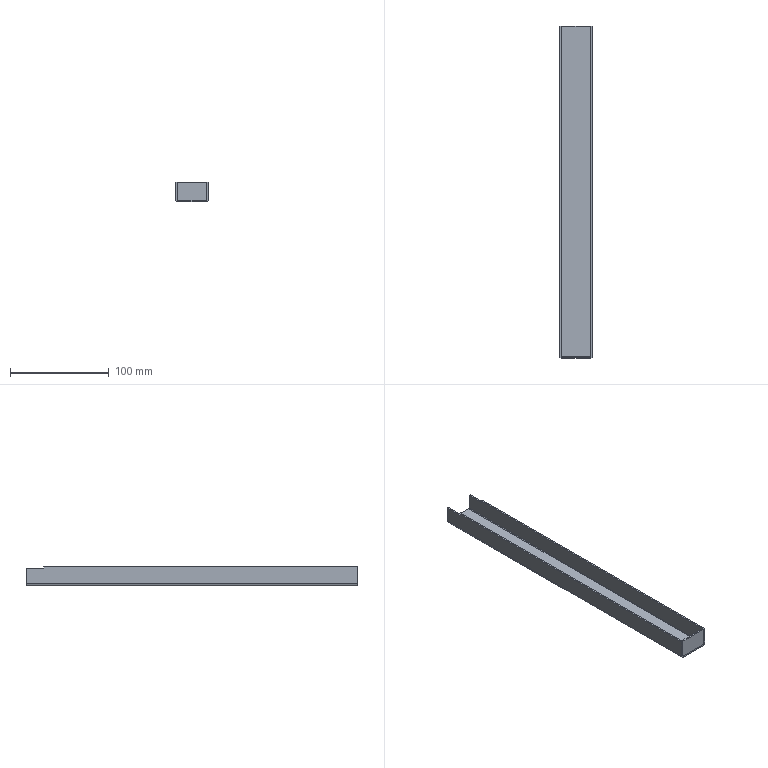Part | SolidWorks | features BaseBody 2 | 2 solids | 34 faces | box 33 x 336 x 20 mm | volume 35464 mm3 | plane 28 | cylinder 6 | commonest cylinder face diameters 1 x4 4 x2
STEP:
#1=CARTESIAN_POINT('',(-15.,150.,18.5));
#2=VERTEX_POINT('',#1);
#3=CARTESIAN_POINT('',(-15.,150.,16.5));
#4=VERTEX_POINT('',#3);
#5=CARTESIAN_POINT('',(-15.,150.,0.));
#6=DIRECTION('',(0.,0.,-1.));
#7=VECTOR('',#6,1000.);
#8=LINE('',#5,#7);
#9=EDGE_CURVE('',#2,#4,#8,.T.);
#10=ORIENTED_EDGE('',*,*,#9,.T.);
#11=CARTESIAN_POINT('',(-16.5,150.,16.5));
#12=VERTEX_POINT('',#11);
#13=CARTESIAN_POINT('',(-16.5,150.,16.5));
#14=DIRECTION('',(1.,0.,0.));
#15=VECTOR('',#14,1000.);
#16=LINE('',#13,#15);
#17=EDGE_CURVE('',#12,#4,#16,.T.);
#18=ORIENTED_EDGE('',*,*,#17,.F.);
#19=CARTESIAN_POINT('',(-16.5,150.,18.5));
#20=VERTEX_POINT('',#19);
#21=CARTESIAN_POINT('',(-16.5,150.,18.5));
#22=DIRECTION('',(0.,0.,-1.));
#23=VECTOR('',#22,1000.);
#24=LINE('',#21,#23);
#25=EDGE_CURVE('',#20,#12,#24,.T.);
#26=ORIENTED_EDGE('',*,*,#25,.F.);
#27=CARTESIAN_POINT('',(-16.5,150.,18.5));
#28=DIRECTION('',(1.,0.,0.));
#29=VECTOR('',#28,1000.);
#30=LINE('',#27,#29);
#31=EDGE_CURVE('',#20,#2,#30,.T.);
#32=ORIENTED_EDGE('',*,*,#31,.T.);
#33=EDGE_LOOP('',(#10,#18,#26,#32));
#34=FACE_OUTER_BOUND('',#33,.T.);
#35=CARTESIAN_POINT('',(-16.5,150.,18.5));
#36=DIRECTION('',(0.,-1.,0.));
#37=DIRECTION('',(0.,0.,-1.));
#38=AXIS2_PLACEMENT_3D('',#35,#36,#37);
#39=PLANE('',#38);
#40=ADVANCED_FACE('',(#34),#39,.F.);
#41=CARTESIAN_POINT('',(-15.,168.,16.5));
#42=VERTEX_POINT('',#41);
#43=CARTESIAN_POINT('',(-15.,0.,16.5));
#44=DIRECTION('',(0.,1.,0.));
#45=VECTOR('',#44,1000.);
#46=LINE('',#43,#45);
#47=EDGE_CURVE('',#4,#42,#46,.T.);
#48=ORIENTED_EDGE('',*,*,#47,.T.);
#49=CARTESIAN_POINT('',(-16.5,168.,16.5));
#50=VERTEX_POINT('',#49);
#51=CARTESIAN_POINT('',(-16.5,168.,16.5));
#52=DIRECTION('',(1.,0.,0.));
#53=VECTOR('',#52,1000.);
#54=LINE('',#51,#53);
#55=EDGE_CURVE('',#50,#42,#54,.T.);
#56=ORIENTED_EDGE('',*,*,#55,.F.);
#57=CARTESIAN_POINT('',(-16.5,168.,16.5));
#58=DIRECTION('',(0.,1.,0.));
#59=VECTOR('',#58,1000.);
#60=LINE('',#57,#59);
#61=EDGE_CURVE('',#12,#50,#60,.T.);
#62=ORIENTED_EDGE('',*,*,#61,.F.);
#63=ORIENTED_EDGE('',*,*,#17,.T.);
#64=EDGE_LOOP('',(#48,#56,#62,#63));
#65=FACE_OUTER_BOUND('',#64,.T.);
#66=CARTESIAN_POINT('',(-16.5,168.,16.5));
#67=DIRECTION('',(0.,0.,-1.));
#68=DIRECTION('',(-1.,0.,0.));
#69=AXIS2_PLACEMENT_3D('',#66,#67,#68);
#70=PLANE('',#69);
#71=ADVANCED_FACE('',(#65),#70,.F.);
#72=CARTESIAN_POINT('',(15.,168.,16.5));
#73=VERTEX_POINT('',#72);
#74=CARTESIAN_POINT('',(15.,150.,16.5));
#75=VERTEX_POINT('',#74);
#76=CARTESIAN_POINT('',(15.,0.,16.5));
#77=DIRECTION('',(0.,-1.,0.));
#78=VECTOR('',#77,1000.);
#79=LINE('',#76,#78);
#80=EDGE_CURVE('',#73,#75,#79,.T.);
#81=ORIENTED_EDGE('',*,*,#80,.T.);
#82=CARTESIAN_POINT('',(16.5,150.,16.5));
#83=VERTEX_POINT('',#82);
#84=CARTESIAN_POINT('',(-16.5,150.,16.5));
#85=DIRECTION('',(1.,0.,0.));
#86=VECTOR('',#85,1000.);
#87=LINE('',#84,#86);
#88=EDGE_CURVE('',#75,#83,#87,.T.);
#89=ORIENTED_EDGE('',*,*,#88,.T.);
#90=CARTESIAN_POINT('',(16.5,168.,16.5));
#91=VERTEX_POINT('',#90);
#92=CARTESIAN_POINT('',(16.5,168.,16.5));
#93=DIRECTION('',(0.,1.,0.));
#94=VECTOR('',#93,1000.);
#95=LINE('',#92,#94);
#96=EDGE_CURVE('',#83,#91,#95,.T.);
#97=ORIENTED_EDGE('',*,*,#96,.T.);
#98=CARTESIAN_POINT('',(-16.5,168.,16.5));
#99=DIRECTION('',(1.,0.,0.));
#100=VECTOR('',#99,1000.);
#101=LINE('',#98,#100);
#102=EDGE_CURVE('',#73,#91,#101,.T.);
#103=ORIENTED_EDGE('',*,*,#102,.F.);
#104=EDGE_LOOP('',(#81,#89,#97,#103));
#105=FACE_OUTER_BOUND('',#104,.T.);
#106=CARTESIAN_POINT('',(-16.5,168.,16.5));
#107=DIRECTION('',(0.,0.,-1.));
#108=DIRECTION('',(-1.,0.,0.));
#109=AXIS2_PLACEMENT_3D('',#106,#107,#108);
#110=PLANE('',#109);
#111=ADVANCED_FACE('',(#105),#110,.F.);
#112=CARTESIAN_POINT('',(15.,150.,18.5));
#113=VERTEX_POINT('',#112);
#114=CARTESIAN_POINT('',(15.,150.,0.));
#115=DIRECTION('',(0.,0.,1.));
#116=VECTOR('',#115,1000.);
#117=LINE('',#114,#116);
#118=EDGE_CURVE('',#75,#113,#117,.T.);
#119=ORIENTED_EDGE('',*,*,#118,.T.);
#120=CARTESIAN_POINT('',(16.5,150.,18.5));
#121=VERTEX_POINT('',#120);
#122=CARTESIAN_POINT('',(16.5,150.,18.5));
#123=DIRECTION('',(-1.,0.,0.));
#124=VECTOR('',#123,1000.);
#125=LINE('',#122,#124);
#126=EDGE_CURVE('',#121,#113,#125,.T.);
#127=ORIENTED_EDGE('',*,*,#126,.F.);
#128=CARTESIAN_POINT('',(16.5,150.,18.5));
#129=DIRECTION('',(0.,0.,-1.));
#130=VECTOR('',#129,1000.);
#131=LINE('',#128,#130);
#132=EDGE_CURVE('',#121,#83,#131,.T.);
#133=ORIENTED_EDGE('',*,*,#132,.T.);
#134=ORIENTED_EDGE('',*,*,#88,.F.);
#135=EDGE_LOOP('',(#119,#127,#133,#134));
#136=FACE_OUTER_BOUND('',#135,.T.);
#137=CARTESIAN_POINT('',(-16.5,150.,18.5));
#138=DIRECTION('',(0.,-1.,0.));
#139=DIRECTION('',(0.,0.,-1.));
#140=AXIS2_PLACEMENT_3D('',#137,#138,#139);
#141=PLANE('',#140);
#142=ADVANCED_FACE('',(#136),#141,.F.);
#143=CARTESIAN_POINT('',(16.5,-168.,18.5));
#144=VERTEX_POINT('',#143);
#145=CARTESIAN_POINT('',(16.5,-168.,18.5));
#146=DIRECTION('',(0.,-1.,0.));
#147=VECTOR('',#146,1000.);
#148=LINE('',#145,#147);
#149=EDGE_CURVE('',#121,#144,#148,.T.);
#150=ORIENTED_EDGE('',*,*,#149,.F.);
#151=ORIENTED_EDGE('',*,*,#126,.T.);
#152=CARTESIAN_POINT('',(15.,-168.,18.5));
#153=VERTEX_POINT('',#152);
#154=CARTESIAN_POINT('',(15.,-168.,18.5));
#155=DIRECTION('',(0.,-1.,0.));
#156=VECTOR('',#155,1000.);
#157=LINE('',#154,#156);
#158=EDGE_CURVE('',#113,#153,#157,.T.);
#159=ORIENTED_EDGE('',*,*,#158,.T.);
#160=CARTESIAN_POINT('',(16.5,-168.,18.5));
#161=DIRECTION('',(-1.,0.,0.));
#162=VECTOR('',#161,1000.);
#163=LINE('',#160,#162);
#164=EDGE_CURVE('',#144,#153,#163,.T.);
#165=ORIENTED_EDGE('',*,*,#164,.F.);
#166=EDGE_LOOP('',(#150,#151,#159,#165));
#167=FACE_OUTER_BOUND('',#166,.T.);
#168=CARTESIAN_POINT('',(16.5,-168.,18.5));
#169=DIRECTION('',(0.,0.,-1.));
#170=DIRECTION('',(-1.,0.,0.));
#171=AXIS2_PLACEMENT_3D('',#168,#169,#170);
#172=PLANE('',#171);
#173=ADVANCED_FACE('',(#167),#172,.F.);
#174=ORIENTED_EDGE('',*,*,#80,.F.);
#175=CARTESIAN_POINT('',(15.,168.,0.5));
#176=VERTEX_POINT('',#175);
#177=CARTESIAN_POINT('',(15.,168.,18.5));
#178=DIRECTION('',(0.,0.,1.));
#179=VECTOR('',#178,1000.);
#180=LINE('',#177,#179);
#181=EDGE_CURVE('',#176,#73,#180,.T.);
#182=ORIENTED_EDGE('',*,*,#181,.F.);
#183=CARTESIAN_POINT('',(15.,-168.,0.5));
#184=VERTEX_POINT('',#183);
#185=CARTESIAN_POINT('',(15.,-168.,0.5));
#186=DIRECTION('',(0.,1.,0.));
#187=VECTOR('',#186,1000.);
#188=LINE('',#185,#187);
#189=EDGE_CURVE('',#184,#176,#188,.T.);
#190=ORIENTED_EDGE('',*,*,#189,.F.);
#191=CARTESIAN_POINT('',(15.,-168.,0.));
#192=DIRECTION('',(0.,0.,-1.));
#193=VECTOR('',#192,1000.);
#194=LINE('',#191,#193);
#195=EDGE_CURVE('',#153,#184,#194,.T.);
#196=ORIENTED_EDGE('',*,*,#195,.F.);
#197=ORIENTED_EDGE('',*,*,#158,.F.);
#198=ORIENTED_EDGE('',*,*,#118,.F.);
#199=EDGE_LOOP('',(#174,#182,#190,#196,#197,#198));
#200=FACE_OUTER_BOUND('',#199,.T.);
#201=CARTESIAN_POINT('',(15.,0.,0.));
#202=DIRECTION('',(-1.,0.,0.));
#203=DIRECTION('',(0.,1.,0.));
#204=AXIS2_PLACEMENT_3D('',#201,#202,#203);
#205=PLANE('',#204);
#206=ADVANCED_FACE('',(#200),#205,.T.);
#207=CARTESIAN_POINT('',(16.5,168.,0.5));
#208=VERTEX_POINT('',#207);
#209=CARTESIAN_POINT('',(16.5,168.,18.5));
#210=DIRECTION('',(0.,0.,1.));
#211=VECTOR('',#210,1000.);
#212=LINE('',#209,#211);
#213=EDGE_CURVE('',#208,#91,#212,.T.);
#214=ORIENTED_EDGE('',*,*,#213,.T.);
#215=ORIENTED_EDGE('',*,*,#96,.F.);
#216=ORIENTED_EDGE('',*,*,#132,.F.);
#217=ORIENTED_EDGE('',*,*,#149,.T.);
#218=CARTESIAN_POINT('',(16.5,-168.,0.5));
#219=VERTEX_POINT('',#218);
#220=CARTESIAN_POINT('',(16.5,-168.,0.));
#221=DIRECTION('',(0.,0.,-1.));
#222=VECTOR('',#221,1000.);
#223=LINE('',#220,#222);
#224=EDGE_CURVE('',#144,#219,#223,.T.);
#225=ORIENTED_EDGE('',*,*,#224,.T.);
#226=CARTESIAN_POINT('',(16.5,0.,0.5));
#227=DIRECTION('',(0.,-1.,0.));
#228=VECTOR('',#227,1000.);
#229=LINE('',#226,#228);
#230=EDGE_CURVE('',#208,#219,#229,.T.);
#231=ORIENTED_EDGE('',*,*,#230,.F.);
#232=EDGE_LOOP('',(#214,#215,#216,#217,#225,#231));
#233=FACE_OUTER_BOUND('',#232,.T.);
#234=CARTESIAN_POINT('',(16.5,0.,0.));
#235=DIRECTION('',(-1.,0.,0.));
#236=DIRECTION('',(0.,1.,0.));
#237=AXIS2_PLACEMENT_3D('',#234,#235,#236);
#238=PLANE('',#237);
#239=ADVANCED_FACE('',(#233),#238,.F.);
#240=ORIENTED_EDGE('',*,*,#181,.T.);
#241=ORIENTED_EDGE('',*,*,#102,.T.);
#242=ORIENTED_EDGE('',*,*,#213,.F.);
#243=CARTESIAN_POINT('',(15.,168.,0.5));
#244=DIRECTION('',(1.,0.,0.));
#245=VECTOR('',#244,1000.);
#246=LINE('',#243,#245);
#247=EDGE_CURVE('',#176,#208,#246,.T.);
#248=ORIENTED_EDGE('',*,*,#247,.F.);
#249=EDGE_LOOP('',(#240,#241,#242,#248));
#250=FACE_OUTER_BOUND('',#249,.T.);
#251=CARTESIAN_POINT('',(16.5,168.,18.5));
#252=DIRECTION('',(0.,-1.,0.));
#253=DIRECTION('',(0.,0.,-1.));
#254=AXIS2_PLACEMENT_3D('',#251,#252,#253);
#255=PLANE('',#254);
#256=ADVANCED_FACE('',(#250),#255,.F.);
#257=CARTESIAN_POINT('',(15.,-168.,0.5));
#258=DIRECTION('',(1.,0.,0.));
#259=VECTOR('',#258,1000.);
#260=LINE('',#257,#259);
#261=EDGE_CURVE('',#184,#219,#260,.T.);
#262=ORIENTED_EDGE('',*,*,#261,.T.);
#263=ORIENTED_EDGE('',*,*,#224,.F.);
#264=ORIENTED_EDGE('',*,*,#164,.T.);
#265=ORIENTED_EDGE('',*,*,#195,.T.);
#266=EDGE_LOOP('',(#262,#263,#264,#265));
#267=FACE_OUTER_BOUND('',#266,.T.);
#268=CARTESIAN_POINT('',(16.5,-168.,0.));
#269=DIRECTION('',(0.,1.,0.));
#270=DIRECTION('',(1.,0.,0.));
#271=AXIS2_PLACEMENT_3D('',#268,#269,#270);
#272=PLANE('',#271);
#273=ADVANCED_FACE('',(#267),#272,.F.);
#274=CARTESIAN_POINT('',(14.5,168.,0.));
#275=VERTEX_POINT('',#274);
#276=CARTESIAN_POINT('',(14.5,-168.,0.));
#277=VERTEX_POINT('',#276);
#278=CARTESIAN_POINT('',(14.5,168.,0.));
#279=DIRECTION('',(0.,-1.,0.));
#280=VECTOR('',#279,1000.);
#281=LINE('',#278,#280);
#282=EDGE_CURVE('',#275,#277,#281,.T.);
#283=ORIENTED_EDGE('',*,*,#282,.T.);
#284=CARTESIAN_POINT('',(14.5,-168.,0.5));
#285=DIRECTION('',(0.,-1.,0.));
#286=DIRECTION('',(0.,0.,1.));
#287=AXIS2_PLACEMENT_3D('',#284,#285,#286);
#288=CIRCLE('',#287,0.5);
#289=EDGE_CURVE('',#277,#184,#288,.T.);
#290=ORIENTED_EDGE('',*,*,#289,.T.);
#291=ORIENTED_EDGE('',*,*,#189,.T.);
#292=CARTESIAN_POINT('',(14.5,168.,0.5));
#293=DIRECTION('',(0.,1.,0.));
#294=DIRECTION('',(0.,0.,1.));
#295=AXIS2_PLACEMENT_3D('',#292,#293,#294);
#296=CIRCLE('',#295,0.5);
#297=EDGE_CURVE('',#176,#275,#296,.T.);
#298=ORIENTED_EDGE('',*,*,#297,.T.);
#299=EDGE_LOOP('',(#283,#290,#291,#298));
#300=FACE_OUTER_BOUND('',#299,.T.);
#301=CARTESIAN_POINT('',(14.5,168.,0.5));
#302=DIRECTION('',(0.,1.,0.));
#303=DIRECTION('',(1.,0.,0.));
#304=AXIS2_PLACEMENT_3D('',#301,#302,#303);
#305=CYLINDRICAL_SURFACE('',#304,0.5);
#306=ADVANCED_FACE('',(#300),#305,.F.);
#307=CARTESIAN_POINT('',(14.5,168.,-1.5));
#308=VERTEX_POINT('',#307);
#309=CARTESIAN_POINT('',(14.5,-168.,-1.5));
#310=VERTEX_POINT('',#309);
#311=CARTESIAN_POINT('',(14.5,168.,-1.5));
#312=DIRECTION('',(0.,-1.,0.));
#313=VECTOR('',#312,1000.);
#314=LINE('',#311,#313);
#315=EDGE_CURVE('',#308,#310,#314,.T.);
#316=ORIENTED_EDGE('',*,*,#315,.F.);
#317=CARTESIAN_POINT('',(14.5,168.,0.5));
#318=DIRECTION('',(0.,1.,0.));
#319=DIRECTION('',(0.,0.,1.));
#320=AXIS2_PLACEMENT_3D('',#317,#318,#319);
#321=CIRCLE('',#320,2.);
#322=EDGE_CURVE('',#208,#308,#321,.T.);
#323=ORIENTED_EDGE('',*,*,#322,.F.);
#324=ORIENTED_EDGE('',*,*,#230,.T.);
#325=CARTESIAN_POINT('',(14.5,-168.,0.5));
#326=DIRECTION('',(0.,-1.,0.));
#327=DIRECTION('',(0.,0.,1.));
#328=AXIS2_PLACEMENT_3D('',#325,#326,#327);
#329=CIRCLE('',#328,2.);
#330=EDGE_CURVE('',#310,#219,#329,.T.);
#331=ORIENTED_EDGE('',*,*,#330,.F.);
#332=EDGE_LOOP('',(#316,#323,#324,#331));
#333=FACE_OUTER_BOUND('',#332,.T.);
#334=CARTESIAN_POINT('',(14.5,168.,0.5));
#335=DIRECTION('',(0.,1.,0.));
#336=DIRECTION('',(1.,0.,0.));
#337=AXIS2_PLACEMENT_3D('',#334,#335,#336);
#338=CYLINDRICAL_SURFACE('',#337,2.);
#339=ADVANCED_FACE('',(#333),#338,.T.);
#340=ORIENTED_EDGE('',*,*,#297,.F.);
#341=ORIENTED_EDGE('',*,*,#247,.T.);
#342=ORIENTED_EDGE('',*,*,#322,.T.);
#343=CARTESIAN_POINT('',(14.5,168.,0.));
#344=DIRECTION('',(0.,0.,-1.));
#345=VECTOR('',#344,1000.);
#346=LINE('',#343,#345);
#347=EDGE_CURVE('',#275,#308,#346,.T.);
#348=ORIENTED_EDGE('',*,*,#347,.F.);
#349=EDGE_LOOP('',(#340,#341,#342,#348));
#350=FACE_OUTER_BOUND('',#349,.T.);
#351=CARTESIAN_POINT('',(14.5,168.,0.5));
#352=DIRECTION('',(0.,-1.,0.));
#353=DIRECTION('',(0.,0.,-1.));
#354=AXIS2_PLACEMENT_3D('',#351,#352,#353);
#355=PLANE('',#354);
#356=ADVANCED_FACE('',(#350),#355,.F.);
#357=ORIENTED_EDGE('',*,*,#261,.F.);
#358=ORIENTED_EDGE('',*,*,#289,.F.);
#359=CARTESIAN_POINT('',(14.5,-168.,0.));
#360=DIRECTION('',(0.,0.,-1.));
#361=VECTOR('',#360,1000.);
#362=LINE('',#359,#361);
#363=EDGE_CURVE('',#277,#310,#362,.T.);
#364=ORIENTED_EDGE('',*,*,#363,.T.);
#365=ORIENTED_EDGE('',*,*,#330,.T.);
#366=EDGE_LOOP('',(#357,#358,#364,#365));
#367=FACE_OUTER_BOUND('',#366,.T.);
#368=CARTESIAN_POINT('',(14.5,-168.,0.5));
#369=DIRECTION('',(0.,-1.,0.));
#370=DIRECTION('',(0.,0.,-1.));
#371=AXIS2_PLACEMENT_3D('',#368,#369,#370);
#372=PLANE('',#371);
#373=ADVANCED_FACE('',(#367),#372,.T.);
#374=CARTESIAN_POINT('',(-15.,-168.,18.5));
#375=VERTEX_POINT('',#374);
#376=CARTESIAN_POINT('',(-15.,168.,18.5));
#377=DIRECTION('',(0.,1.,0.));
#378=VECTOR('',#377,1000.);
#379=LINE('',#376,#378);
#380=EDGE_CURVE('',#375,#2,#379,.T.);
#381=ORIENTED_EDGE('',*,*,#380,.T.);
#382=ORIENTED_EDGE('',*,*,#31,.F.);
#383=CARTESIAN_POINT('',(-16.5,-168.,18.5));
#384=VERTEX_POINT('',#383);
#385=CARTESIAN_POINT('',(-16.5,168.,18.5));
#386=DIRECTION('',(0.,1.,0.));
#387=VECTOR('',#386,1000.);
#388=LINE('',#385,#387);
#389=EDGE_CURVE('',#384,#20,#388,.T.);
#390=ORIENTED_EDGE('',*,*,#389,.F.);
#391=CARTESIAN_POINT('',(-16.5,-168.,18.5));
#392=DIRECTION('',(1.,0.,0.));
#393=VECTOR('',#392,1000.);
#394=LINE('',#391,#393);
#395=EDGE_CURVE('',#384,#375,#394,.T.);
#396=ORIENTED_EDGE('',*,*,#395,.T.);
#397=EDGE_LOOP('',(#381,#382,#390,#396));
#398=FACE_OUTER_BOUND('',#397,.T.);
#399=CARTESIAN_POINT('',(-16.5,168.,18.5));
#400=DIRECTION('',(0.,0.,-1.));
#401=DIRECTION('',(0.,-1.,0.));
#402=AXIS2_PLACEMENT_3D('',#399,#400,#401);
#403=PLANE('',#402);
#404=ADVANCED_FACE('',(#398),#403,.F.);
#405=ORIENTED_EDGE('',*,*,#47,.F.);
#406=ORIENTED_EDGE('',*,*,#9,.F.);
#407=ORIENTED_EDGE('',*,*,#380,.F.);
#408=CARTESIAN_POINT('',(-15.,-168.,0.5));
#409=VERTEX_POINT('',#408);
#410=CARTESIAN_POINT('',(-15.,-168.,18.5));
#411=DIRECTION('',(0.,0.,1.));
#412=VECTOR('',#411,1000.);
#413=LINE('',#410,#412);
#414=EDGE_CURVE('',#409,#375,#413,.T.);
#415=ORIENTED_EDGE('',*,*,#414,.F.);
#416=CARTESIAN_POINT('',(-15.,168.,0.5));
#417=VERTEX_POINT('',#416);
#418=CARTESIAN_POINT('',(-15.,168.,0.5));
#419=DIRECTION('',(0.,-1.,0.));
#420=VECTOR('',#419,1000.);
#421=LINE('',#418,#420);
#422=EDGE_CURVE('',#417,#409,#421,.T.);
#423=ORIENTED_EDGE('',*,*,#422,.F.);
#424=CARTESIAN_POINT('',(-15.,168.,0.));
#425=DIRECTION('',(0.,0.,-1.));
#426=VECTOR('',#425,1000.);
#427=LINE('',#424,#426);
#428=EDGE_CURVE('',#42,#417,#427,.T.);
#429=ORIENTED_EDGE('',*,*,#428,.F.);
#430=EDGE_LOOP('',(#405,#406,#407,#415,#423,#429));
#431=FACE_OUTER_BOUND('',#430,.T.);
#432=CARTESIAN_POINT('',(-15.,0.,0.));
#433=DIRECTION('',(1.,0.,0.));
#434=DIRECTION('',(0.,0.,1.));
#435=AXIS2_PLACEMENT_3D('',#432,#433,#434);
#436=PLANE('',#435);
#437=ADVANCED_FACE('',(#431),#436,.T.);
#438=ORIENTED_EDGE('',*,*,#25,.T.);
#439=ORIENTED_EDGE('',*,*,#61,.T.);
#440=CARTESIAN_POINT('',(-16.5,168.,0.5));
#441=VERTEX_POINT('',#440);
#442=CARTESIAN_POINT('',(-16.5,168.,0.));
#443=DIRECTION('',(0.,0.,-1.));
#444=VECTOR('',#443,1000.);
#445=LINE('',#442,#444);
#446=EDGE_CURVE('',#50,#441,#445,.T.);
#447=ORIENTED_EDGE('',*,*,#446,.T.);
#448=CARTESIAN_POINT('',(-16.5,-168.,0.5));
#449=VERTEX_POINT('',#448);
#450=CARTESIAN_POINT('',(-16.5,0.,0.5));
#451=DIRECTION('',(0.,1.,0.));
#452=VECTOR('',#451,1000.);
#453=LINE('',#450,#452);
#454=EDGE_CURVE('',#449,#441,#453,.T.);
#455=ORIENTED_EDGE('',*,*,#454,.F.);
#456=CARTESIAN_POINT('',(-16.5,-168.,18.5));
#457=DIRECTION('',(0.,0.,1.));
#458=VECTOR('',#457,1000.);
#459=LINE('',#456,#458);
#460=EDGE_CURVE('',#449,#384,#459,.T.);
#461=ORIENTED_EDGE('',*,*,#460,.T.);
#462=ORIENTED_EDGE('',*,*,#389,.T.);
#463=EDGE_LOOP('',(#438,#439,#447,#455,#461,#462));
#464=FACE_OUTER_BOUND('',#463,.T.);
#465=CARTESIAN_POINT('',(-16.5,0.,0.));
#466=DIRECTION('',(1.,0.,0.));
#467=DIRECTION('',(0.,0.,1.));
#468=AXIS2_PLACEMENT_3D('',#465,#466,#467);
#469=PLANE('',#468);
#470=ADVANCED_FACE('',(#464),#469,.F.);
#471=ORIENTED_EDGE('',*,*,#446,.F.);
#472=ORIENTED_EDGE('',*,*,#55,.T.);
#473=ORIENTED_EDGE('',*,*,#428,.T.);
#474=CARTESIAN_POINT('',(-15.,168.,0.5));
#475=DIRECTION('',(-1.,0.,0.));
#476=VECTOR('',#475,1000.);
#477=LINE('',#474,#476);
#478=EDGE_CURVE('',#417,#441,#477,.T.);
#479=ORIENTED_EDGE('',*,*,#478,.T.);
#480=EDGE_LOOP('',(#471,#472,#473,#479));
#481=FACE_OUTER_BOUND('',#480,.T.);
#482=CARTESIAN_POINT('',(-16.5,168.,0.));
#483=DIRECTION('',(0.,-1.,0.));
#484=DIRECTION('',(0.,0.,-1.));
#485=AXIS2_PLACEMENT_3D('',#482,#483,#484);
#486=PLANE('',#485);
#487=ADVANCED_FACE('',(#481),#486,.F.);
#488=CARTESIAN_POINT('',(-15.,-168.,0.5));
#489=DIRECTION('',(-1.,0.,0.));
#490=VECTOR('',#489,1000.);
#491=LINE('',#488,#490);
#492=EDGE_CURVE('',#409,#449,#491,.T.);
#493=ORIENTED_EDGE('',*,*,#492,.F.);
#494=ORIENTED_EDGE('',*,*,#414,.T.);
#495=ORIENTED_EDGE('',*,*,#395,.F.);
#496=ORIENTED_EDGE('',*,*,#460,.F.);
#497=EDGE_LOOP('',(#493,#494,#495,#496));
#498=FACE_OUTER_BOUND('',#497,.T.);
#499=CARTESIAN_POINT('',(-16.5,-168.,18.5));
#500=DIRECTION('',(0.,1.,0.));
#501=DIRECTION('',(1.,0.,0.));
#502=AXIS2_PLACEMENT_3D('',#499,#500,#501);
#503=PLANE('',#502);
#504=ADVANCED_FACE('',(#498),#503,.F.);
#505=CARTESIAN_POINT('',(-14.5,-168.,0.));
#506=VERTEX_POINT('',#505);
#507=CARTESIAN_POINT('',(-14.5,168.,0.));
#508=VERTEX_POINT('',#507);
#509=CARTESIAN_POINT('',(-14.5,-168.,0.));
#510=DIRECTION('',(0.,1.,0.));
#511=VECTOR('',#510,1000.);
#512=LINE('',#509,#511);
#513=EDGE_CURVE('',#506,#508,#512,.T.);
#514=ORIENTED_EDGE('',*,*,#513,.T.);
#515=CARTESIAN_POINT('',(-14.5,168.,0.5));
#516=DIRECTION('',(0.,1.,0.));
#517=DIRECTION('',(0.,0.,-1.));
#518=AXIS2_PLACEMENT_3D('',#515,#516,#517);
#519=CIRCLE('',#518,0.5);
#520=EDGE_CURVE('',#508,#417,#519,.T.);
#521=ORIENTED_EDGE('',*,*,#520,.T.);
#522=ORIENTED_EDGE('',*,*,#422,.T.);
#523=CARTESIAN_POINT('',(-14.5,-168.,0.5));
#524=DIRECTION('',(0.,-1.,0.));
#525=DIRECTION('',(0.,0.,-1.));
#526=AXIS2_PLACEMENT_3D('',#523,#524,#525);
#527=CIRCLE('',#526,0.5);
#528=EDGE_CURVE('',#409,#506,#527,.T.);
#529=ORIENTED_EDGE('',*,*,#528,.T.);
#530=EDGE_LOOP('',(#514,#521,#522,#529));
#531=FACE_OUTER_BOUND('',#530,.T.);
#532=CARTESIAN_POINT('',(-14.5,-168.,0.5));
#533=DIRECTION('',(0.,-1.,0.));
#534=DIRECTION('',(-1.,0.,0.));
#535=AXIS2_PLACEMENT_3D('',#532,#533,#534);
#536=CYLINDRICAL_SURFACE('',#535,0.5);
#537=ADVANCED_FACE('',(#531),#536,.F.);
#538=CARTESIAN_POINT('',(-14.5,-168.,-1.5));
#539=VERTEX_POINT('',#538);
#540=CARTESIAN_POINT('',(-14.5,168.,-1.5));
#541=VERTEX_POINT('',#540);
#542=CARTESIAN_POINT('',(-14.5,-168.,-1.5));
#543=DIRECTION('',(0.,1.,0.));
#544=VECTOR('',#543,1000.);
#545=LINE('',#542,#544);
#546=EDGE_CURVE('',#539,#541,#545,.T.);
#547=ORIENTED_EDGE('',*,*,#546,.F.);
#548=CARTESIAN_POINT('',(-14.5,-168.,0.5));
#549=DIRECTION('',(0.,-1.,0.));
#550=DIRECTION('',(0.,0.,-1.));
#551=AXIS2_PLACEMENT_3D('',#548,#549,#550);
#552=CIRCLE('',#551,2.);
#553=EDGE_CURVE('',#449,#539,#552,.T.);
#554=ORIENTED_EDGE('',*,*,#553,.F.);
#555=ORIENTED_EDGE('',*,*,#454,.T.);
#556=CARTESIAN_POINT('',(-14.5,168.,0.5));
#557=DIRECTION('',(0.,1.,0.));
#558=DIRECTION('',(0.,0.,-1.));
#559=AXIS2_PLACEMENT_3D('',#556,#557,#558);
#560=CIRCLE('',#559,2.);
#561=EDGE_CURVE('',#541,#441,#560,.T.);
#562=ORIENTED_EDGE('',*,*,#561,.F.);
#563=EDGE_LOOP('',(#547,#554,#555,#562));
#564=FACE_OUTER_BOUND('',#563,.T.);
#565=CARTESIAN_POINT('',(-14.5,-168.,0.5));
#566=DIRECTION('',(0.,-1.,0.));
#567=DIRECTION('',(-1.,0.,0.));
#568=AXIS2_PLACEMENT_3D('',#565,#566,#567);
#569=CYLINDRICAL_SURFACE('',#568,2.);
#570=ADVANCED_FACE('',(#564),#569,.T.);
#571=ORIENTED_EDGE('',*,*,#528,.F.);
#572=ORIENTED_EDGE('',*,*,#492,.T.);
#573=ORIENTED_EDGE('',*,*,#553,.T.);
#574=CARTESIAN_POINT('',(-14.5,-168.,0.));
#575=DIRECTION('',(0.,0.,-1.));
#576=VECTOR('',#575,1000.);
#577=LINE('',#574,#576);
#578=EDGE_CURVE('',#506,#539,#577,.T.);
#579=ORIENTED_EDGE('',*,*,#578,.F.);
#580=EDGE_LOOP('',(#571,#572,#573,#579));
#581=FACE_OUTER_BOUND('',#580,.T.);
#582=CARTESIAN_POINT('',(-14.5,-168.,0.5));
#583=DIRECTION('',(0.,1.,0.));
#584=DIRECTION('',(1.,0.,0.));
#585=AXIS2_PLACEMENT_3D('',#582,#583,#584);
#586=PLANE('',#585);
#587=ADVANCED_FACE('',(#581),#586,.F.);
#588=ORIENTED_EDGE('',*,*,#478,.F.);
#589=ORIENTED_EDGE('',*,*,#520,.F.);
#590=CARTESIAN_POINT('',(-14.5,168.,0.));
#591=DIRECTION('',(0.,0.,-1.));
#592=VECTOR('',#591,1000.);
#593=LINE('',#590,#592);
#594=EDGE_CURVE('',#508,#541,#593,.T.);
#595=ORIENTED_EDGE('',*,*,#594,.T.);
#596=ORIENTED_EDGE('',*,*,#561,.T.);
#597=EDGE_LOOP('',(#588,#589,#595,#596));
#598=FACE_OUTER_BOUND('',#597,.T.);
#599=CARTESIAN_POINT('',(-14.5,168.,0.5));
#600=DIRECTION('',(0.,1.,0.));
#601=DIRECTION('',(1.,0.,0.));
#602=AXIS2_PLACEMENT_3D('',#599,#600,#601);
#603=PLANE('',#602);
#604=ADVANCED_FACE('',(#598),#603,.T.);
#605=ORIENTED_EDGE('',*,*,#363,.F.);
#606=CARTESIAN_POINT('',(15.,-168.,0.));
#607=DIRECTION('',(1.,0.,0.));
#608=VECTOR('',#607,1000.);
#609=LINE('',#606,#608);
#610=EDGE_CURVE('',#506,#277,#609,.T.);
#611=ORIENTED_EDGE('',*,*,#610,.F.);
#612=ORIENTED_EDGE('',*,*,#578,.T.);
#613=CARTESIAN_POINT('',(15.,-168.,-1.5));
#614=DIRECTION('',(1.,0.,0.));
#615=VECTOR('',#614,1000.);
#616=LINE('',#613,#615);
#617=EDGE_CURVE('',#539,#310,#616,.T.);
#618=ORIENTED_EDGE('',*,*,#617,.T.);
#619=EDGE_LOOP('',(#605,#611,#612,#618));
#620=FACE_OUTER_BOUND('',#619,.T.);
#621=CARTESIAN_POINT('',(15.,-168.,-1.5));
#622=DIRECTION('',(0.,-1.,0.));
#623=DIRECTION('',(0.,0.,-1.));
#624=AXIS2_PLACEMENT_3D('',#621,#622,#623);
#625=PLANE('',#624);
#626=ADVANCED_FACE('',(#620),#625,.T.);
#627=CARTESIAN_POINT('',(15.,168.,0.));
#628=DIRECTION('',(-1.,0.,0.));
#629=VECTOR('',#628,1000.);
#630=LINE('',#627,#629);
#631=EDGE_CURVE('',#275,#508,#630,.T.);
#632=ORIENTED_EDGE('',*,*,#631,.F.);
#633=ORIENTED_EDGE('',*,*,#347,.T.);
#634=CARTESIAN_POINT('',(15.,168.,-1.5));
#635=DIRECTION('',(-1.,0.,0.));
#636=VECTOR('',#635,1000.);
#637=LINE('',#634,#636);
#638=EDGE_CURVE('',#308,#541,#637,.T.);
#639=ORIENTED_EDGE('',*,*,#638,.T.);
#640=ORIENTED_EDGE('',*,*,#594,.F.);
#641=EDGE_LOOP('',(#632,#633,#639,#640));
#642=FACE_OUTER_BOUND('',#641,.T.);
#643=CARTESIAN_POINT('',(15.,168.,-1.5));
#644=DIRECTION('',(0.,1.,0.));
#645=DIRECTION('',(1.,0.,0.));
#646=AXIS2_PLACEMENT_3D('',#643,#644,#645);
#647=PLANE('',#646);
#648=ADVANCED_FACE('',(#642),#647,.T.);
#649=ORIENTED_EDGE('',*,*,#282,.F.);
#650=ORIENTED_EDGE('',*,*,#631,.T.);
#651=ORIENTED_EDGE('',*,*,#513,.F.);
#652=ORIENTED_EDGE('',*,*,#610,.T.);
#653=EDGE_LOOP('',(#649,#650,#651,#652));
#654=FACE_OUTER_BOUND('',#653,.T.);
#655=CARTESIAN_POINT('',(0.,0.,0.));
#656=DIRECTION('',(0.,0.,-1.));
#657=DIRECTION('',(0.,-1.,0.));
#658=AXIS2_PLACEMENT_3D('',#655,#656,#657);
#659=PLANE('',#658);
#660=ADVANCED_FACE('',(#654),#659,.F.);
#661=ORIENTED_EDGE('',*,*,#638,.F.);
#662=ORIENTED_EDGE('',*,*,#315,.T.);
#663=ORIENTED_EDGE('',*,*,#617,.F.);
#664=ORIENTED_EDGE('',*,*,#546,.T.);
#665=EDGE_LOOP('',(#661,#662,#663,#664));
#666=FACE_OUTER_BOUND('',#665,.T.);
#667=CARTESIAN_POINT('',(0.,0.,-1.5));
#668=DIRECTION('',(0.,0.,-1.));
#669=DIRECTION('',(0.,-1.,0.));
#670=AXIS2_PLACEMENT_3D('',#667,#668,#669);
#671=PLANE('',#670);
#672=ADVANCED_FACE('',(#666),#671,.T.);
#673=CLOSED_SHELL('',(#40,#71,#111,#142,#173,#206,#239,#256,#273,#306,#339,#356,#373,#404,#437,#470,#487,#504,#537,#570,#587,#604,#626,#648,#660,#672));
#674=MANIFOLD_SOLID_BREP('',#673);
#675=CARTESIAN_POINT('',(15.,-168.,18.5));
#676=VERTEX_POINT('',#675);
#677=CARTESIAN_POINT('',(-15.,-168.,18.5));
#678=VERTEX_POINT('',#677);
#679=CARTESIAN_POINT('',(-15.,-168.,18.5));
#680=DIRECTION('',(-1.,0.,0.));
#681=VECTOR('',#680,1000.);
#682=LINE('',#679,#681);
#683=EDGE_CURVE('',#676,#678,#682,.T.);
#684=ORIENTED_EDGE('',*,*,#683,.T.);
#685=CARTESIAN_POINT('',(-15.,-168.,0.5));
#686=VERTEX_POINT('',#685);
#687=CARTESIAN_POINT('',(-15.,-168.,0.5));
#688=DIRECTION('',(0.,0.,-1.));
#689=VECTOR('',#688,1000.);
#690=LINE('',#687,#689);
#691=EDGE_CURVE('',#678,#686,#690,.T.);
#692=ORIENTED_EDGE('',*,*,#691,.T.);
#693=CARTESIAN_POINT('',(-14.5,-168.,0.));
#694=VERTEX_POINT('',#693);
#695=CARTESIAN_POINT('',(-14.5,-168.,0.5));
#696=DIRECTION('',(0.,-1.,0.));
#697=DIRECTION('',(1.,0.,0.));
#698=AXIS2_PLACEMENT_3D('',#695,#696,#697);
#699=CIRCLE('',#698,0.5);
#700=EDGE_CURVE('',#686,#694,#699,.T.);
#701=ORIENTED_EDGE('',*,*,#700,.T.);
#702=CARTESIAN_POINT('',(14.5,-168.,0.));
#703=VERTEX_POINT('',#702);
#704=CARTESIAN_POINT('',(-14.5,-168.,0.));
#705=DIRECTION('',(1.,0.,0.));
#706=VECTOR('',#705,1000.);
#707=LINE('',#704,#706);
#708=EDGE_CURVE('',#694,#703,#707,.T.);
#709=ORIENTED_EDGE('',*,*,#708,.T.);
#710=CARTESIAN_POINT('',(15.,-168.,0.5));
#711=VERTEX_POINT('',#710);
#712=CARTESIAN_POINT('',(14.5,-168.,0.5));
#713=DIRECTION('',(0.,-1.,0.));
#714=DIRECTION('',(1.,0.,0.));
#715=AXIS2_PLACEMENT_3D('',#712,#713,#714);
#716=CIRCLE('',#715,0.5);
#717=EDGE_CURVE('',#703,#711,#716,.T.);
#718=ORIENTED_EDGE('',*,*,#717,.T.);
#719=CARTESIAN_POINT('',(15.,-168.,18.5));
#720=DIRECTION('',(0.,0.,1.));
#721=VECTOR('',#720,1000.);
#722=LINE('',#719,#721);
#723=EDGE_CURVE('',#711,#676,#722,.T.);
#724=ORIENTED_EDGE('',*,*,#723,.T.);
#725=EDGE_LOOP('',(#684,#692,#701,#709,#718,#724));
#726=FACE_OUTER_BOUND('',#725,.T.);
#727=CARTESIAN_POINT('',(14.5,-168.,0.5));
#728=DIRECTION('',(0.,-1.,0.));
#729=DIRECTION('',(0.,0.,-1.));
#730=AXIS2_PLACEMENT_3D('',#727,#728,#729);
#731=PLANE('',#730);
#732=ADVANCED_FACE('',(#726),#731,.T.);
#733=CARTESIAN_POINT('',(15.,-166.5,18.5));
#734=VERTEX_POINT('',#733);
#735=CARTESIAN_POINT('',(-15.,-166.5,18.5));
#736=VERTEX_POINT('',#735);
#737=CARTESIAN_POINT('',(-15.,-166.5,18.5));
#738=DIRECTION('',(-1.,0.,0.));
#739=VECTOR('',#738,1000.);
#740=LINE('',#737,#739);
#741=EDGE_CURVE('',#734,#736,#740,.T.);
#742=ORIENTED_EDGE('',*,*,#741,.F.);
#743=CARTESIAN_POINT('',(15.,-166.5,0.5));
#744=VERTEX_POINT('',#743);
#745=CARTESIAN_POINT('',(15.,-166.5,18.5));
#746=DIRECTION('',(0.,0.,1.));
#747=VECTOR('',#746,1000.);
#748=LINE('',#745,#747);
#749=EDGE_CURVE('',#744,#734,#748,.T.);
#750=ORIENTED_EDGE('',*,*,#749,.F.);
#751=CARTESIAN_POINT('',(14.5,-166.5,0.));
#752=VERTEX_POINT('',#751);
#753=CARTESIAN_POINT('',(14.5,-166.5,0.5));
#754=DIRECTION('',(0.,-1.,0.));
#755=DIRECTION('',(1.,0.,0.));
#756=AXIS2_PLACEMENT_3D('',#753,#754,#755);
#757=CIRCLE('',#756,0.5);
#758=EDGE_CURVE('',#752,#744,#757,.T.);
#759=ORIENTED_EDGE('',*,*,#758,.F.);
#760=CARTESIAN_POINT('',(-14.5,-166.5,0.));
#761=VERTEX_POINT('',#760);
#762=CARTESIAN_POINT('',(-14.5,-166.5,0.));
#763=DIRECTION('',(1.,0.,0.));
#764=VECTOR('',#763,1000.);
#765=LINE('',#762,#764);
#766=EDGE_CURVE('',#761,#752,#765,.T.);
#767=ORIENTED_EDGE('',*,*,#766,.F.);
#768=CARTESIAN_POINT('',(-15.,-166.5,0.5));
#769=VERTEX_POINT('',#768);
#770=CARTESIAN_POINT('',(-14.5,-166.5,0.5));
#771=DIRECTION('',(0.,-1.,0.));
#772=DIRECTION('',(1.,0.,0.));
#773=AXIS2_PLACEMENT_3D('',#770,#771,#772);
#774=CIRCLE('',#773,0.5);
#775=EDGE_CURVE('',#769,#761,#774,.T.);
#776=ORIENTED_EDGE('',*,*,#775,.F.);
#777=CARTESIAN_POINT('',(-15.,-166.5,0.5));
#778=DIRECTION('',(0.,0.,-1.));
#779=VECTOR('',#778,1000.);
#780=LINE('',#777,#779);
#781=EDGE_CURVE('',#736,#769,#780,.T.);
#782=ORIENTED_EDGE('',*,*,#781,.F.);
#783=EDGE_LOOP('',(#742,#750,#759,#767,#776,#782));
#784=FACE_OUTER_BOUND('',#783,.T.);
#785=CARTESIAN_POINT('',(14.5,-166.5,0.5));
#786=DIRECTION('',(0.,-1.,0.));
#787=DIRECTION('',(0.,0.,-1.));
#788=AXIS2_PLACEMENT_3D('',#785,#786,#787);
#789=PLANE('',#788);
#790=ADVANCED_FACE('',(#784),#789,.F.);
#791=ORIENTED_EDGE('',*,*,#691,.F.);
#792=CARTESIAN_POINT('',(-15.,-166.5,18.5));
#793=DIRECTION('',(0.,-1.,0.));
#794=VECTOR('',#793,1000.);
#795=LINE('',#792,#794);
#796=EDGE_CURVE('',#736,#678,#795,.T.);
#797=ORIENTED_EDGE('',*,*,#796,.F.);
#798=ORIENTED_EDGE('',*,*,#781,.T.);
#799=CARTESIAN_POINT('',(-15.,-166.5,0.5));
#800=DIRECTION('',(0.,-1.,0.));
#801=VECTOR('',#800,1000.);
#802=LINE('',#799,#801);
#803=EDGE_CURVE('',#769,#686,#802,.T.);
#804=ORIENTED_EDGE('',*,*,#803,.T.);
#805=EDGE_LOOP('',(#791,#797,#798,#804));
#806=FACE_OUTER_BOUND('',#805,.T.);
#807=CARTESIAN_POINT('',(-15.,-166.5,0.5));
#808=DIRECTION('',(-1.,0.,0.));
#809=DIRECTION('',(0.,0.,1.));
#810=AXIS2_PLACEMENT_3D('',#807,#808,#809);
#811=PLANE('',#810);
#812=ADVANCED_FACE('',(#806),#811,.T.);
#813=ORIENTED_EDGE('',*,*,#700,.F.);
#814=ORIENTED_EDGE('',*,*,#803,.F.);
#815=ORIENTED_EDGE('',*,*,#775,.T.);
#816=CARTESIAN_POINT('',(-14.5,-166.5,0.));
#817=DIRECTION('',(0.,-1.,0.));
#818=VECTOR('',#817,1000.);
#819=LINE('',#816,#818);
#820=EDGE_CURVE('',#761,#694,#819,.T.);
#821=ORIENTED_EDGE('',*,*,#820,.T.);
#822=EDGE_LOOP('',(#813,#814,#815,#821));
#823=FACE_OUTER_BOUND('',#822,.T.);
#824=CARTESIAN_POINT('',(-14.5,-166.5,0.5));
#825=DIRECTION('',(0.,-1.,0.));
#826=DIRECTION('',(1.,0.,0.));
#827=AXIS2_PLACEMENT_3D('',#824,#825,#826);
#828=CYLINDRICAL_SURFACE('',#827,0.5);
#829=ADVANCED_FACE('',(#823),#828,.T.);
#830=ORIENTED_EDGE('',*,*,#708,.F.);
#831=ORIENTED_EDGE('',*,*,#820,.F.);
#832=ORIENTED_EDGE('',*,*,#766,.T.);
#833=CARTESIAN_POINT('',(14.5,-166.5,0.));
#834=DIRECTION('',(0.,-1.,0.));
#835=VECTOR('',#834,1000.);
#836=LINE('',#833,#835);
#837=EDGE_CURVE('',#752,#703,#836,.T.);
#838=ORIENTED_EDGE('',*,*,#837,.T.);
#839=EDGE_LOOP('',(#830,#831,#832,#838));
#840=FACE_OUTER_BOUND('',#839,.T.);
#841=CARTESIAN_POINT('',(-14.5,-166.5,0.));
#842=DIRECTION('',(0.,0.,-1.));
#843=DIRECTION('',(0.,-1.,0.));
#844=AXIS2_PLACEMENT_3D('',#841,#842,#843);
#845=PLANE('',#844);
#846=ADVANCED_FACE('',(#840),#845,.T.);
#847=ORIENTED_EDGE('',*,*,#717,.F.);
#848=ORIENTED_EDGE('',*,*,#837,.F.);
#849=ORIENTED_EDGE('',*,*,#758,.T.);
#850=CARTESIAN_POINT('',(15.,-166.5,0.5));
#851=DIRECTION('',(0.,-1.,0.));
#852=VECTOR('',#851,1000.);
#853=LINE('',#850,#852);
#854=EDGE_CURVE('',#744,#711,#853,.T.);
#855=ORIENTED_EDGE('',*,*,#854,.T.);
#856=EDGE_LOOP('',(#847,#848,#849,#855));
#857=FACE_OUTER_BOUND('',#856,.T.);
#858=CARTESIAN_POINT('',(14.5,-166.5,0.5));
#859=DIRECTION('',(0.,-1.,0.));
#860=DIRECTION('',(1.,0.,0.));
#861=AXIS2_PLACEMENT_3D('',#858,#859,#860);
#862=CYLINDRICAL_SURFACE('',#861,0.5);
#863=ADVANCED_FACE('',(#857),#862,.T.);
#864=ORIENTED_EDGE('',*,*,#723,.F.);
#865=ORIENTED_EDGE('',*,*,#854,.F.);
#866=ORIENTED_EDGE('',*,*,#749,.T.);
#867=CARTESIAN_POINT('',(15.,-166.5,18.5));
#868=DIRECTION('',(0.,-1.,0.));
#869=VECTOR('',#868,1000.);
#870=LINE('',#867,#869);
#871=EDGE_CURVE('',#734,#676,#870,.T.);
#872=ORIENTED_EDGE('',*,*,#871,.T.);
#873=EDGE_LOOP('',(#864,#865,#866,#872));
#874=FACE_OUTER_BOUND('',#873,.T.);
#875=CARTESIAN_POINT('',(15.,-166.5,18.5));
#876=DIRECTION('',(1.,0.,0.));
#877=DIRECTION('',(0.,0.,-1.));
#878=AXIS2_PLACEMENT_3D('',#875,#876,#877);
#879=PLANE('',#878);
#880=ADVANCED_FACE('',(#874),#879,.T.);
#881=ORIENTED_EDGE('',*,*,#683,.F.);
#882=ORIENTED_EDGE('',*,*,#871,.F.);
#883=ORIENTED_EDGE('',*,*,#741,.T.);
#884=ORIENTED_EDGE('',*,*,#796,.T.);
#885=EDGE_LOOP('',(#881,#882,#883,#884));
#886=FACE_OUTER_BOUND('',#885,.T.);
#887=CARTESIAN_POINT('',(-15.,-166.5,18.5));
#888=DIRECTION('',(0.,0.,1.));
#889=DIRECTION('',(0.,-1.,0.));
#890=AXIS2_PLACEMENT_3D('',#887,#888,#889);
#891=PLANE('',#890);
#892=ADVANCED_FACE('',(#886),#891,.T.);
#893=CLOSED_SHELL('',(#732,#790,#812,#829,#846,#863,#880,#892));
#894=MANIFOLD_SOLID_BREP('',#893);
#895=CARTESIAN_POINT('',(0.,0.,0.));
#896=DIRECTION('',(0.,0.,1.));
#897=DIRECTION('',(1.,0.,0.));
#898=AXIS2_PLACEMENT_3D('',#895,#896,#897);
#899=(LENGTH_UNIT()NAMED_UNIT(*)SI_UNIT(.MILLI.,.METRE.));
#900=UNCERTAINTY_MEASURE_WITH_UNIT(LENGTH_MEASURE(0.00001),#899,'','');
#901=(NAMED_UNIT(*)PLANE_ANGLE_UNIT()SI_UNIT($,.RADIAN.));
#902=(NAMED_UNIT(*)SI_UNIT($,.STERADIAN.)SOLID_ANGLE_UNIT());
#903=(GEOMETRIC_REPRESENTATION_CONTEXT(3)GLOBAL_UNCERTAINTY_ASSIGNED_CONTEXT((#900))GLOBAL_UNIT_ASSIGNED_CONTEXT((#899,#901,#902))REPRESENTATION_CONTEXT('',''));
#904=ADVANCED_BREP_SHAPE_REPRESENTATION('',(#674,#894,#898),#903);